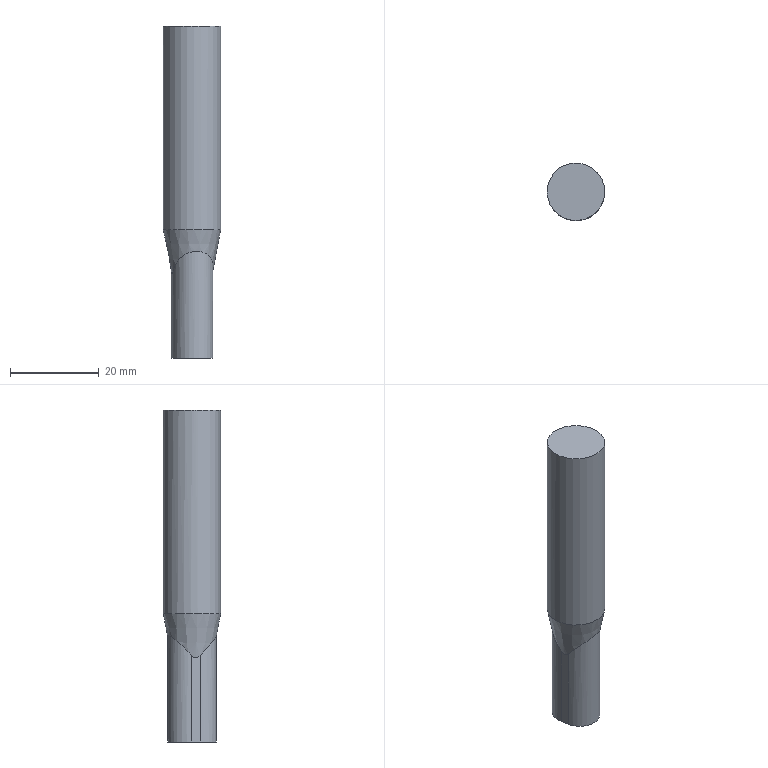Part | NX | features solid 2 | 1 solid | 8 faces | box 13 x 13 x 75 mm | volume 8694 mm3 | plane 4 | cylinder 3 | cone 1 | commonest cylinder face diameters 9.1 x2 13 x1
STEP:
#1=CARTESIAN_POINT('',(800.65,-3.029,65.557));
#2=VERTEX_POINT('',#1);
#3=CARTESIAN_POINT('',(801.036,-4.992,65.557));
#4=VERTEX_POINT('',#3);
#5=CARTESIAN_POINT('',(800.65,-3.029,65.557));
#6=CARTESIAN_POINT('',(800.701,-3.289,65.265));
#7=CARTESIAN_POINT('',(800.842,-4.009,64.735));
#8=CARTESIAN_POINT('',(800.984,-4.731,65.265));
#9=CARTESIAN_POINT('',(801.036,-4.992,65.557));
#10=B_SPLINE_CURVE_WITH_KNOTS('',3,(#5,#6,#7,#8,#9),.UNSPECIFIED.,.F.,.F.,(4,1,4),(0.000000301,0.001176,0.002351),.UNSPECIFIED.);
#11=EDGE_CURVE('',#2,#4,#10,.T.);
#12=ORIENTED_EDGE('',*,*,#11,.T.);
#13=CARTESIAN_POINT('',(801.036,-4.992,46.));
#14=VERTEX_POINT('',#13);
#15=CARTESIAN_POINT('',(801.036,-4.992,46.));
#16=DIRECTION('',(0.,0.,1.));
#17=VECTOR('',#16,1000.);
#18=LINE('',#15,#17);
#19=EDGE_CURVE('',#14,#4,#18,.T.);
#20=ORIENTED_EDGE('',*,*,#19,.F.);
#21=CARTESIAN_POINT('',(800.65,-3.029,46.));
#22=VERTEX_POINT('',#21);
#23=CARTESIAN_POINT('',(800.843,-4.01,46.));
#24=DIRECTION('',(0.193,-0.9812,0.));
#25=VECTOR('',#24,1000.);
#26=LINE('',#23,#25);
#27=EDGE_CURVE('',#22,#14,#26,.T.);
#28=ORIENTED_EDGE('',*,*,#27,.F.);
#29=CARTESIAN_POINT('',(800.65,-3.029,46.));
#30=DIRECTION('',(0.,0.,1.));
#31=VECTOR('',#30,1000.);
#32=LINE('',#29,#31);
#33=EDGE_CURVE('',#22,#2,#32,.T.);
#34=ORIENTED_EDGE('',*,*,#33,.T.);
#35=EDGE_LOOP('',(#12,#20,#28,#34));
#36=FACE_BOUND('',#35,.T.);
#37=CARTESIAN_POINT('',(800.843,-4.01,46.));
#38=DIRECTION('',(0.9812,0.193,0.));
#39=DIRECTION('',(0.,0.,1.));
#40=AXIS2_PLACEMENT_3D('',#37,#38,#39);
#41=PLANE('',#40);
#42=ADVANCED_FACE('',(#36),#41,.T.);
#43=ORIENTED_EDGE('',*,*,#27,.T.);
#44=CARTESIAN_POINT('',(792.107,-6.748,46.));
#45=VERTEX_POINT('',#44);
#46=CARTESIAN_POINT('',(796.571,-5.87,46.));
#47=DIRECTION('',(0.,0.,-1.));
#48=DIRECTION('',(-0.9812,-0.193,0.));
#49=AXIS2_PLACEMENT_3D('',#46,#47,#48);
#50=CIRCLE('',#49,4.55);
#51=EDGE_CURVE('',#14,#45,#50,.T.);
#52=ORIENTED_EDGE('',*,*,#51,.T.);
#53=CARTESIAN_POINT('',(791.721,-4.786,46.));
#54=VERTEX_POINT('',#53);
#55=CARTESIAN_POINT('',(791.914,-5.767,46.));
#56=DIRECTION('',(-0.193,0.9812,0.));
#57=VECTOR('',#56,1000.);
#58=LINE('',#55,#57);
#59=EDGE_CURVE('',#45,#54,#58,.T.);
#60=ORIENTED_EDGE('',*,*,#59,.T.);
#61=CARTESIAN_POINT('',(796.185,-3.907,46.));
#62=DIRECTION('',(0.,0.,-1.));
#63=DIRECTION('',(-0.9812,-0.193,0.));
#64=AXIS2_PLACEMENT_3D('',#61,#62,#63);
#65=CIRCLE('',#64,4.55);
#66=EDGE_CURVE('',#54,#22,#65,.T.);
#67=ORIENTED_EDGE('',*,*,#66,.T.);
#68=EDGE_LOOP('',(#43,#52,#60,#67));
#69=FACE_BOUND('',#68,.T.);
#70=CARTESIAN_POINT('',(796.378,-4.889,46.));
#71=DIRECTION('',(0.,0.,-1.));
#72=DIRECTION('',(0.9812,0.193,0.));
#73=AXIS2_PLACEMENT_3D('',#70,#71,#72);
#74=PLANE('',#73);
#75=ADVANCED_FACE('',(#69),#74,.T.);
#76=CARTESIAN_POINT('',(792.107,-6.748,65.557));
#77=VERTEX_POINT('',#76);
#78=CARTESIAN_POINT('',(791.721,-4.786,65.557));
#79=VERTEX_POINT('',#78);
#80=CARTESIAN_POINT('',(792.107,-6.748,65.557));
#81=CARTESIAN_POINT('',(792.056,-6.488,65.265));
#82=CARTESIAN_POINT('',(791.914,-5.768,64.735));
#83=CARTESIAN_POINT('',(791.772,-5.046,65.265));
#84=CARTESIAN_POINT('',(791.721,-4.786,65.557));
#85=B_SPLINE_CURVE_WITH_KNOTS('',3,(#80,#81,#82,#83,#84),.UNSPECIFIED.,.F.,.F.,(4,1,4),(0.000000301,0.001176,0.002351),.UNSPECIFIED.);
#86=EDGE_CURVE('',#77,#79,#85,.T.);
#87=ORIENTED_EDGE('',*,*,#86,.T.);
#88=CARTESIAN_POINT('',(791.721,-4.786,46.));
#89=DIRECTION('',(0.,0.,1.));
#90=VECTOR('',#89,1000.);
#91=LINE('',#88,#90);
#92=EDGE_CURVE('',#54,#79,#91,.T.);
#93=ORIENTED_EDGE('',*,*,#92,.F.);
#94=ORIENTED_EDGE('',*,*,#59,.F.);
#95=CARTESIAN_POINT('',(792.107,-6.748,46.));
#96=DIRECTION('',(0.,0.,1.));
#97=VECTOR('',#96,1000.);
#98=LINE('',#95,#97);
#99=EDGE_CURVE('',#45,#77,#98,.T.);
#100=ORIENTED_EDGE('',*,*,#99,.T.);
#101=EDGE_LOOP('',(#87,#93,#94,#100));
#102=FACE_BOUND('',#101,.T.);
#103=CARTESIAN_POINT('',(791.914,-5.767,46.));
#104=DIRECTION('',(-0.9812,-0.193,0.));
#105=DIRECTION('',(0.,0.,-1.));
#106=AXIS2_PLACEMENT_3D('',#103,#104,#105);
#107=PLANE('',#106);
#108=ADVANCED_FACE('',(#102),#107,.T.);
#109=CARTESIAN_POINT('',(800.65,-3.029,65.557));
#110=CARTESIAN_POINT('',(800.556,-2.552,66.092));
#111=CARTESIAN_POINT('',(800.216,-1.615,67.141));
#112=CARTESIAN_POINT('',(799.173,-0.3308,68.604));
#113=CARTESIAN_POINT('',(797.511,0.6063,69.782));
#114=CARTESIAN_POINT('',(795.281,0.7433,70.301));
#115=CARTESIAN_POINT('',(793.249,-0.2289,69.785));
#116=CARTESIAN_POINT('',(792.068,-1.726,68.606));
#117=CARTESIAN_POINT('',(791.587,-3.304,67.148));
#118=CARTESIAN_POINT('',(791.627,-4.307,66.093));
#119=CARTESIAN_POINT('',(791.721,-4.786,65.557));
#120=B_SPLINE_CURVE_WITH_KNOTS('',3,(#109,#110,#111,#112,#113,#114,#115,#116,#117,#118,#119),.UNSPECIFIED.,.F.,.F.,(4,1,1,1,1,1,1,1,4),(0.0007425,0.002903,0.005063,0.007223,0.009383,0.01154,0.0137,0.01586,0.01802),.UNSPECIFIED.);
#121=EDGE_CURVE('',#2,#79,#120,.T.);
#122=ORIENTED_EDGE('',*,*,#121,.T.);
#123=ORIENTED_EDGE('',*,*,#86,.F.);
#124=CARTESIAN_POINT('',(792.107,-6.748,65.557));
#125=CARTESIAN_POINT('',(792.201,-7.225,66.092));
#126=CARTESIAN_POINT('',(792.54,-8.162,67.141));
#127=CARTESIAN_POINT('',(793.583,-9.446,68.604));
#128=CARTESIAN_POINT('',(795.245,-10.383,69.782));
#129=CARTESIAN_POINT('',(797.476,-10.52,70.301));
#130=CARTESIAN_POINT('',(799.507,-9.548,69.785));
#131=CARTESIAN_POINT('',(800.688,-8.051,68.606));
#132=CARTESIAN_POINT('',(801.17,-6.473,67.148));
#133=CARTESIAN_POINT('',(801.13,-5.47,66.093));
#134=CARTESIAN_POINT('',(801.036,-4.992,65.557));
#135=B_SPLINE_CURVE_WITH_KNOTS('',3,(#124,#125,#126,#127,#128,#129,#130,#131,#132,#133,#134),.UNSPECIFIED.,.F.,.F.,(4,1,1,1,1,1,1,1,4),(0.0007425,0.002903,0.005063,0.007223,0.009383,0.01154,0.0137,0.01586,0.01802),.UNSPECIFIED.);
#136=EDGE_CURVE('',#77,#4,#135,.T.);
#137=ORIENTED_EDGE('',*,*,#136,.T.);
#138=ORIENTED_EDGE('',*,*,#11,.F.);
#139=EDGE_LOOP('',(#122,#123,#137,#138));
#140=FACE_BOUND('',#139,.T.);
#141=CARTESIAN_POINT('',(790.,-6.143,75.));
#142=VERTEX_POINT('',#141);
#143=CARTESIAN_POINT('',(796.378,-4.889,75.));
#144=DIRECTION('',(0.,0.,-1.));
#145=DIRECTION('',(-0.9812,-0.193,0.));
#146=AXIS2_PLACEMENT_3D('',#143,#144,#145);
#147=CIRCLE('',#146,6.5);
#148=EDGE_CURVE('',#142,#142,#147,.T.);
#149=ORIENTED_EDGE('',*,*,#148,.T.);
#150=EDGE_LOOP('',(#149));
#151=FACE_BOUND('',#150,.T.);
#152=CARTESIAN_POINT('',(796.378,-4.889,65.));
#153=DIRECTION('',(0.,0.,1.));
#154=DIRECTION('',(-0.9812,-0.193,0.));
#155=AXIS2_PLACEMENT_3D('',#152,#153,#154);
#156=CONICAL_SURFACE('',#155,4.55,0.1926);
#157=ADVANCED_FACE('',(#140,#151),#156,.T.);
#158=CARTESIAN_POINT('',(789.878,-4.889,121.));
#159=VERTEX_POINT('',#158);
#160=CARTESIAN_POINT('',(796.378,-4.889,121.));
#161=DIRECTION('',(0.,0.,-1.));
#162=DIRECTION('',(-1.,0.,0.));
#163=AXIS2_PLACEMENT_3D('',#160,#161,#162);
#164=CIRCLE('',#163,6.5);
#165=EDGE_CURVE('',#159,#159,#164,.F.);
#166=ORIENTED_EDGE('',*,*,#165,.T.);
#167=EDGE_LOOP('',(#166));
#168=FACE_BOUND('',#167,.T.);
#169=CARTESIAN_POINT('',(796.378,-4.889,121.));
#170=DIRECTION('',(0.,0.,1.));
#171=DIRECTION('',(-0.9812,-0.193,0.));
#172=AXIS2_PLACEMENT_3D('',#169,#170,#171);
#173=PLANE('',#172);
#174=ADVANCED_FACE('',(#168),#173,.T.);
#175=ORIENTED_EDGE('',*,*,#165,.F.);
#176=EDGE_LOOP('',(#175));
#177=FACE_BOUND('',#176,.T.);
#178=ORIENTED_EDGE('',*,*,#148,.F.);
#179=EDGE_LOOP('',(#178));
#180=FACE_BOUND('',#179,.T.);
#181=CARTESIAN_POINT('',(796.378,-4.889,75.));
#182=DIRECTION('',(0.,0.,1.));
#183=DIRECTION('',(-0.9812,-0.193,0.));
#184=AXIS2_PLACEMENT_3D('',#181,#182,#183);
#185=CYLINDRICAL_SURFACE('',#184,6.5);
#186=ADVANCED_FACE('',(#177,#180),#185,.T.);
#187=ORIENTED_EDGE('',*,*,#19,.T.);
#188=ORIENTED_EDGE('',*,*,#136,.F.);
#189=ORIENTED_EDGE('',*,*,#99,.F.);
#190=ORIENTED_EDGE('',*,*,#51,.F.);
#191=EDGE_LOOP('',(#187,#188,#189,#190));
#192=FACE_BOUND('',#191,.T.);
#193=CARTESIAN_POINT('',(796.571,-5.87,46.));
#194=DIRECTION('',(0.,0.,1.));
#195=DIRECTION('',(-0.9812,-0.193,0.));
#196=AXIS2_PLACEMENT_3D('',#193,#194,#195);
#197=CYLINDRICAL_SURFACE('',#196,4.55);
#198=ADVANCED_FACE('',(#192),#197,.T.);
#199=ORIENTED_EDGE('',*,*,#66,.F.);
#200=ORIENTED_EDGE('',*,*,#92,.T.);
#201=ORIENTED_EDGE('',*,*,#121,.F.);
#202=ORIENTED_EDGE('',*,*,#33,.F.);
#203=EDGE_LOOP('',(#199,#200,#201,#202));
#204=FACE_BOUND('',#203,.T.);
#205=CARTESIAN_POINT('',(796.185,-3.907,46.));
#206=DIRECTION('',(0.,0.,1.));
#207=DIRECTION('',(-0.9812,-0.193,0.));
#208=AXIS2_PLACEMENT_3D('',#205,#206,#207);
#209=CYLINDRICAL_SURFACE('',#208,4.55);
#210=ADVANCED_FACE('',(#204),#209,.T.);
#211=CLOSED_SHELL('',(#42,#75,#108,#157,#174,#186,#198,#210));
#212=MANIFOLD_SOLID_BREP('',#211);
#213=(LENGTH_UNIT()NAMED_UNIT(*)SI_UNIT(.MILLI.,.METRE.));
#214=UNCERTAINTY_MEASURE_WITH_UNIT(LENGTH_MEASURE(0.0508),#213,'','');
#215=(NAMED_UNIT(*)PLANE_ANGLE_UNIT()SI_UNIT($,.RADIAN.));
#216=(NAMED_UNIT(*)SI_UNIT($,.STERADIAN.)SOLID_ANGLE_UNIT());
#217=(GEOMETRIC_REPRESENTATION_CONTEXT(3)GLOBAL_UNCERTAINTY_ASSIGNED_CONTEXT((#214))GLOBAL_UNIT_ASSIGNED_CONTEXT((#213,#215,#216))REPRESENTATION_CONTEXT('',''));
#218=ADVANCED_BREP_SHAPE_REPRESENTATION('',(#212),#217);